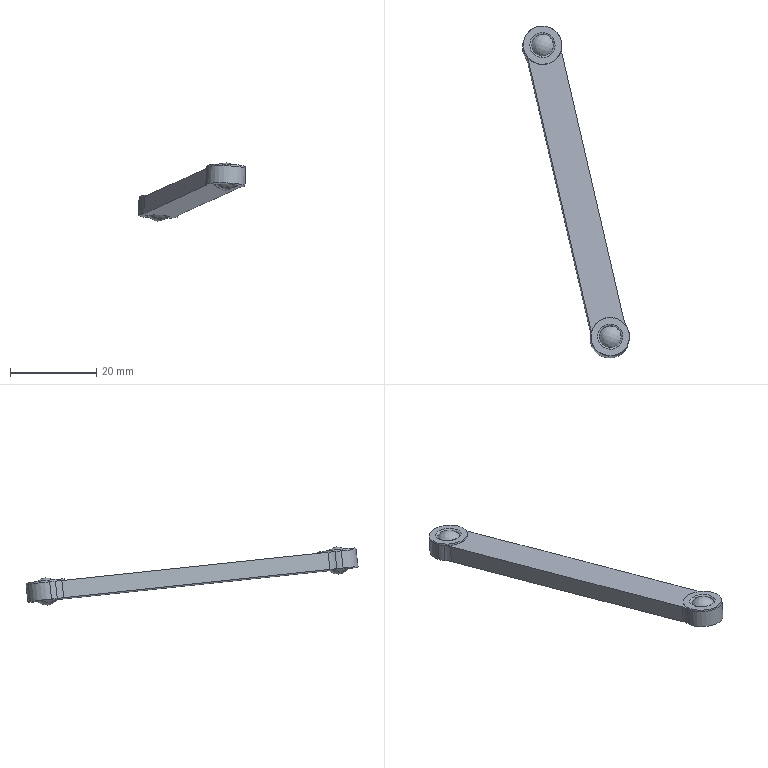Part | STEP file | Zaokr_glenie2 | 1 solid | 28 faces | box 24.844 x 77.037 x 13.475 mm | volume 2577 mm3 | spline 10 | cylinder 10 | plane 6 | torus 2 | commonest cylinder face diameters 9 x4 10 x4 5.5 x2